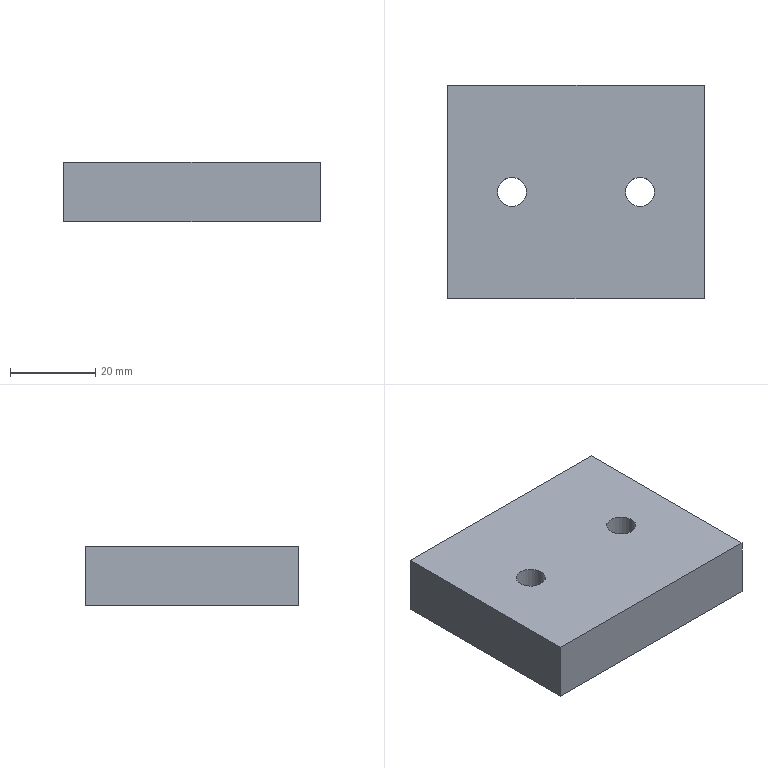Part | SolidWorks | features Extrusion 1, HoleWzd 1 | 1 solid | 10 faces | box 60 x 50 x 14 mm | volume 40983 mm3 | plane 6 | cylinder 4 | commonest cylinder face diameters 6.8 x4
STEP:
#1=CARTESIAN_POINT('',(-18.4,0.,0.));
#2=VERTEX_POINT('',#1);
#3=CARTESIAN_POINT('',(-11.6,0.,0.));
#4=VERTEX_POINT('',#3);
#5=CARTESIAN_POINT('',(-15.,0.,0.));
#6=DIRECTION('',(0.,0.,1.));
#7=DIRECTION('',(1.,0.,0.));
#8=AXIS2_PLACEMENT_3D('',#5,#6,#7);
#9=CIRCLE('',#8,3.4);
#10=EDGE_CURVE('',#2,#4,#9,.T.);
#11=ORIENTED_EDGE('',*,*,#10,.F.);
#12=CARTESIAN_POINT('',(-18.4,0.,14.));
#13=VERTEX_POINT('',#12);
#14=CARTESIAN_POINT('',(-18.4,0.,14.));
#15=DIRECTION('',(0.,0.,1.));
#16=VECTOR('',#15,1000.);
#17=LINE('',#14,#16);
#18=EDGE_CURVE('',#2,#13,#17,.T.);
#19=ORIENTED_EDGE('',*,*,#18,.T.);
#20=CARTESIAN_POINT('',(-11.6,0.,14.));
#21=VERTEX_POINT('',#20);
#22=CARTESIAN_POINT('',(-15.,0.,14.));
#23=DIRECTION('',(0.,0.,1.));
#24=DIRECTION('',(1.,0.,0.));
#25=AXIS2_PLACEMENT_3D('',#22,#23,#24);
#26=CIRCLE('',#25,3.4);
#27=EDGE_CURVE('',#13,#21,#26,.T.);
#28=ORIENTED_EDGE('',*,*,#27,.T.);
#29=CARTESIAN_POINT('',(-11.6,0.,14.));
#30=DIRECTION('',(0.,0.,1.));
#31=VECTOR('',#30,1000.);
#32=LINE('',#29,#31);
#33=EDGE_CURVE('',#4,#21,#32,.T.);
#34=ORIENTED_EDGE('',*,*,#33,.F.);
#35=EDGE_LOOP('',(#11,#19,#28,#34));
#36=FACE_OUTER_BOUND('',#35,.T.);
#37=CARTESIAN_POINT('',(-15.,0.,14.));
#38=DIRECTION('',(0.,0.,1.));
#39=DIRECTION('',(1.,0.,0.));
#40=AXIS2_PLACEMENT_3D('',#37,#38,#39);
#41=CYLINDRICAL_SURFACE('',#40,3.4);
#42=ADVANCED_FACE('',(#36),#41,.F.);
#43=CARTESIAN_POINT('',(11.6,0.,0.));
#44=VERTEX_POINT('',#43);
#45=CARTESIAN_POINT('',(18.4,0.,0.));
#46=VERTEX_POINT('',#45);
#47=CARTESIAN_POINT('',(15.,0.,0.));
#48=DIRECTION('',(0.,0.,1.));
#49=DIRECTION('',(1.,0.,0.));
#50=AXIS2_PLACEMENT_3D('',#47,#48,#49);
#51=CIRCLE('',#50,3.4);
#52=EDGE_CURVE('',#44,#46,#51,.T.);
#53=ORIENTED_EDGE('',*,*,#52,.F.);
#54=CARTESIAN_POINT('',(11.6,0.,14.));
#55=VERTEX_POINT('',#54);
#56=CARTESIAN_POINT('',(11.6,0.,14.));
#57=DIRECTION('',(0.,0.,1.));
#58=VECTOR('',#57,1000.);
#59=LINE('',#56,#58);
#60=EDGE_CURVE('',#44,#55,#59,.T.);
#61=ORIENTED_EDGE('',*,*,#60,.T.);
#62=CARTESIAN_POINT('',(18.4,0.,14.));
#63=VERTEX_POINT('',#62);
#64=CARTESIAN_POINT('',(15.,0.,14.));
#65=DIRECTION('',(0.,0.,1.));
#66=DIRECTION('',(1.,0.,0.));
#67=AXIS2_PLACEMENT_3D('',#64,#65,#66);
#68=CIRCLE('',#67,3.4);
#69=EDGE_CURVE('',#55,#63,#68,.T.);
#70=ORIENTED_EDGE('',*,*,#69,.T.);
#71=CARTESIAN_POINT('',(18.4,0.,14.));
#72=DIRECTION('',(0.,0.,1.));
#73=VECTOR('',#72,1000.);
#74=LINE('',#71,#73);
#75=EDGE_CURVE('',#46,#63,#74,.T.);
#76=ORIENTED_EDGE('',*,*,#75,.F.);
#77=EDGE_LOOP('',(#53,#61,#70,#76));
#78=FACE_OUTER_BOUND('',#77,.T.);
#79=CARTESIAN_POINT('',(15.,0.,14.));
#80=DIRECTION('',(0.,0.,1.));
#81=DIRECTION('',(1.,0.,0.));
#82=AXIS2_PLACEMENT_3D('',#79,#80,#81);
#83=CYLINDRICAL_SURFACE('',#82,3.4);
#84=ADVANCED_FACE('',(#78),#83,.F.);
#85=CARTESIAN_POINT('',(30.,-25.,0.));
#86=VERTEX_POINT('',#85);
#87=CARTESIAN_POINT('',(30.,25.,0.));
#88=VERTEX_POINT('',#87);
#89=CARTESIAN_POINT('',(30.,25.,0.));
#90=DIRECTION('',(0.,1.,0.));
#91=VECTOR('',#90,1000.);
#92=LINE('',#89,#91);
#93=EDGE_CURVE('',#86,#88,#92,.T.);
#94=ORIENTED_EDGE('',*,*,#93,.T.);
#95=CARTESIAN_POINT('',(30.,25.,14.));
#96=VERTEX_POINT('',#95);
#97=CARTESIAN_POINT('',(30.,25.,14.));
#98=DIRECTION('',(0.,0.,-1.));
#99=VECTOR('',#98,1000.);
#100=LINE('',#97,#99);
#101=EDGE_CURVE('',#96,#88,#100,.T.);
#102=ORIENTED_EDGE('',*,*,#101,.F.);
#103=CARTESIAN_POINT('',(30.,-25.,14.));
#104=VERTEX_POINT('',#103);
#105=CARTESIAN_POINT('',(30.,25.,14.));
#106=DIRECTION('',(0.,1.,0.));
#107=VECTOR('',#106,1000.);
#108=LINE('',#105,#107);
#109=EDGE_CURVE('',#104,#96,#108,.T.);
#110=ORIENTED_EDGE('',*,*,#109,.F.);
#111=CARTESIAN_POINT('',(30.,-25.,14.));
#112=DIRECTION('',(0.,0.,-1.));
#113=VECTOR('',#112,1000.);
#114=LINE('',#111,#113);
#115=EDGE_CURVE('',#104,#86,#114,.T.);
#116=ORIENTED_EDGE('',*,*,#115,.T.);
#117=EDGE_LOOP('',(#94,#102,#110,#116));
#118=FACE_OUTER_BOUND('',#117,.T.);
#119=CARTESIAN_POINT('',(30.,25.,14.));
#120=DIRECTION('',(-1.,0.,0.));
#121=DIRECTION('',(0.,-1.,0.));
#122=AXIS2_PLACEMENT_3D('',#119,#120,#121);
#123=PLANE('',#122);
#124=ADVANCED_FACE('',(#118),#123,.F.);
#125=CARTESIAN_POINT('',(-30.,25.,0.));
#126=VERTEX_POINT('',#125);
#127=CARTESIAN_POINT('',(-30.,25.,0.));
#128=DIRECTION('',(-1.,0.,0.));
#129=VECTOR('',#128,1000.);
#130=LINE('',#127,#129);
#131=EDGE_CURVE('',#88,#126,#130,.T.);
#132=ORIENTED_EDGE('',*,*,#131,.T.);
#133=CARTESIAN_POINT('',(-30.,25.,14.));
#134=VERTEX_POINT('',#133);
#135=CARTESIAN_POINT('',(-30.,25.,14.));
#136=DIRECTION('',(0.,0.,-1.));
#137=VECTOR('',#136,1000.);
#138=LINE('',#135,#137);
#139=EDGE_CURVE('',#134,#126,#138,.T.);
#140=ORIENTED_EDGE('',*,*,#139,.F.);
#141=CARTESIAN_POINT('',(-30.,25.,14.));
#142=DIRECTION('',(-1.,0.,0.));
#143=VECTOR('',#142,1000.);
#144=LINE('',#141,#143);
#145=EDGE_CURVE('',#96,#134,#144,.T.);
#146=ORIENTED_EDGE('',*,*,#145,.F.);
#147=ORIENTED_EDGE('',*,*,#101,.T.);
#148=EDGE_LOOP('',(#132,#140,#146,#147));
#149=FACE_OUTER_BOUND('',#148,.T.);
#150=CARTESIAN_POINT('',(-30.,25.,14.));
#151=DIRECTION('',(0.,-1.,0.));
#152=DIRECTION('',(0.,0.,-1.));
#153=AXIS2_PLACEMENT_3D('',#150,#151,#152);
#154=PLANE('',#153);
#155=ADVANCED_FACE('',(#149),#154,.F.);
#156=CARTESIAN_POINT('',(-30.,-25.,0.));
#157=VERTEX_POINT('',#156);
#158=CARTESIAN_POINT('',(-30.,25.,0.));
#159=DIRECTION('',(0.,-1.,0.));
#160=VECTOR('',#159,1000.);
#161=LINE('',#158,#160);
#162=EDGE_CURVE('',#126,#157,#161,.T.);
#163=ORIENTED_EDGE('',*,*,#162,.T.);
#164=CARTESIAN_POINT('',(-30.,-25.,14.));
#165=VERTEX_POINT('',#164);
#166=CARTESIAN_POINT('',(-30.,-25.,14.));
#167=DIRECTION('',(0.,0.,-1.));
#168=VECTOR('',#167,1000.);
#169=LINE('',#166,#168);
#170=EDGE_CURVE('',#165,#157,#169,.T.);
#171=ORIENTED_EDGE('',*,*,#170,.F.);
#172=CARTESIAN_POINT('',(-30.,25.,14.));
#173=DIRECTION('',(0.,-1.,0.));
#174=VECTOR('',#173,1000.);
#175=LINE('',#172,#174);
#176=EDGE_CURVE('',#134,#165,#175,.T.);
#177=ORIENTED_EDGE('',*,*,#176,.F.);
#178=ORIENTED_EDGE('',*,*,#139,.T.);
#179=EDGE_LOOP('',(#163,#171,#177,#178));
#180=FACE_OUTER_BOUND('',#179,.T.);
#181=CARTESIAN_POINT('',(-30.,25.,14.));
#182=DIRECTION('',(1.,0.,0.));
#183=DIRECTION('',(0.,1.,0.));
#184=AXIS2_PLACEMENT_3D('',#181,#182,#183);
#185=PLANE('',#184);
#186=ADVANCED_FACE('',(#180),#185,.F.);
#187=CARTESIAN_POINT('',(-30.,-25.,0.));
#188=DIRECTION('',(1.,0.,0.));
#189=VECTOR('',#188,1000.);
#190=LINE('',#187,#189);
#191=EDGE_CURVE('',#157,#86,#190,.T.);
#192=ORIENTED_EDGE('',*,*,#191,.T.);
#193=ORIENTED_EDGE('',*,*,#115,.F.);
#194=CARTESIAN_POINT('',(-30.,-25.,14.));
#195=DIRECTION('',(1.,0.,0.));
#196=VECTOR('',#195,1000.);
#197=LINE('',#194,#196);
#198=EDGE_CURVE('',#165,#104,#197,.T.);
#199=ORIENTED_EDGE('',*,*,#198,.F.);
#200=ORIENTED_EDGE('',*,*,#170,.T.);
#201=EDGE_LOOP('',(#192,#193,#199,#200));
#202=FACE_OUTER_BOUND('',#201,.T.);
#203=CARTESIAN_POINT('',(-30.,-25.,14.));
#204=DIRECTION('',(0.,1.,0.));
#205=DIRECTION('',(0.,0.,1.));
#206=AXIS2_PLACEMENT_3D('',#203,#204,#205);
#207=PLANE('',#206);
#208=ADVANCED_FACE('',(#202),#207,.F.);
#209=CARTESIAN_POINT('',(-15.,0.,14.));
#210=DIRECTION('',(0.,0.,1.));
#211=DIRECTION('',(1.,0.,0.));
#212=AXIS2_PLACEMENT_3D('',#209,#210,#211);
#213=CIRCLE('',#212,3.4);
#214=EDGE_CURVE('',#21,#13,#213,.T.);
#215=ORIENTED_EDGE('',*,*,#214,.F.);
#216=ORIENTED_EDGE('',*,*,#27,.F.);
#217=EDGE_LOOP('',(#215,#216));
#218=FACE_BOUND('',#217,.T.);
#219=CARTESIAN_POINT('',(15.,0.,14.));
#220=DIRECTION('',(0.,0.,1.));
#221=DIRECTION('',(1.,0.,0.));
#222=AXIS2_PLACEMENT_3D('',#219,#220,#221);
#223=CIRCLE('',#222,3.4);
#224=EDGE_CURVE('',#63,#55,#223,.T.);
#225=ORIENTED_EDGE('',*,*,#224,.F.);
#226=ORIENTED_EDGE('',*,*,#69,.F.);
#227=EDGE_LOOP('',(#225,#226));
#228=FACE_BOUND('',#227,.T.);
#229=ORIENTED_EDGE('',*,*,#109,.T.);
#230=ORIENTED_EDGE('',*,*,#145,.T.);
#231=ORIENTED_EDGE('',*,*,#176,.T.);
#232=ORIENTED_EDGE('',*,*,#198,.T.);
#233=EDGE_LOOP('',(#229,#230,#231,#232));
#234=FACE_OUTER_BOUND('',#233,.T.);
#235=CARTESIAN_POINT('',(0.,0.,14.));
#236=DIRECTION('',(0.,0.,1.));
#237=DIRECTION('',(1.,0.,0.));
#238=AXIS2_PLACEMENT_3D('',#235,#236,#237);
#239=PLANE('',#238);
#240=ADVANCED_FACE('',(#218,#228,#234),#239,.T.);
#241=CARTESIAN_POINT('',(-15.,0.,0.));
#242=DIRECTION('',(0.,0.,1.));
#243=DIRECTION('',(1.,0.,0.));
#244=AXIS2_PLACEMENT_3D('',#241,#242,#243);
#245=CIRCLE('',#244,3.4);
#246=EDGE_CURVE('',#4,#2,#245,.T.);
#247=ORIENTED_EDGE('',*,*,#246,.T.);
#248=ORIENTED_EDGE('',*,*,#10,.T.);
#249=EDGE_LOOP('',(#247,#248));
#250=FACE_BOUND('',#249,.T.);
#251=CARTESIAN_POINT('',(15.,0.,0.));
#252=DIRECTION('',(0.,0.,1.));
#253=DIRECTION('',(1.,0.,0.));
#254=AXIS2_PLACEMENT_3D('',#251,#252,#253);
#255=CIRCLE('',#254,3.4);
#256=EDGE_CURVE('',#46,#44,#255,.T.);
#257=ORIENTED_EDGE('',*,*,#256,.T.);
#258=ORIENTED_EDGE('',*,*,#52,.T.);
#259=EDGE_LOOP('',(#257,#258));
#260=FACE_BOUND('',#259,.T.);
#261=ORIENTED_EDGE('',*,*,#93,.F.);
#262=ORIENTED_EDGE('',*,*,#191,.F.);
#263=ORIENTED_EDGE('',*,*,#162,.F.);
#264=ORIENTED_EDGE('',*,*,#131,.F.);
#265=EDGE_LOOP('',(#261,#262,#263,#264));
#266=FACE_OUTER_BOUND('',#265,.T.);
#267=CARTESIAN_POINT('',(0.,0.,0.));
#268=DIRECTION('',(0.,0.,1.));
#269=DIRECTION('',(1.,0.,0.));
#270=AXIS2_PLACEMENT_3D('',#267,#268,#269);
#271=PLANE('',#270);
#272=ADVANCED_FACE('',(#250,#260,#266),#271,.F.);
#273=ORIENTED_EDGE('',*,*,#60,.F.);
#274=ORIENTED_EDGE('',*,*,#256,.F.);
#275=ORIENTED_EDGE('',*,*,#75,.T.);
#276=ORIENTED_EDGE('',*,*,#224,.T.);
#277=EDGE_LOOP('',(#273,#274,#275,#276));
#278=FACE_OUTER_BOUND('',#277,.T.);
#279=CARTESIAN_POINT('',(15.,0.,14.));
#280=DIRECTION('',(0.,0.,1.));
#281=DIRECTION('',(1.,0.,0.));
#282=AXIS2_PLACEMENT_3D('',#279,#280,#281);
#283=CYLINDRICAL_SURFACE('',#282,3.4);
#284=ADVANCED_FACE('',(#278),#283,.F.);
#285=ORIENTED_EDGE('',*,*,#18,.F.);
#286=ORIENTED_EDGE('',*,*,#246,.F.);
#287=ORIENTED_EDGE('',*,*,#33,.T.);
#288=ORIENTED_EDGE('',*,*,#214,.T.);
#289=EDGE_LOOP('',(#285,#286,#287,#288));
#290=FACE_OUTER_BOUND('',#289,.T.);
#291=CARTESIAN_POINT('',(-15.,0.,14.));
#292=DIRECTION('',(0.,0.,1.));
#293=DIRECTION('',(1.,0.,0.));
#294=AXIS2_PLACEMENT_3D('',#291,#292,#293);
#295=CYLINDRICAL_SURFACE('',#294,3.4);
#296=ADVANCED_FACE('',(#290),#295,.F.);
#297=CLOSED_SHELL('',(#42,#84,#124,#155,#186,#208,#240,#272,#284,#296));
#298=MANIFOLD_SOLID_BREP('',#297);
#299=CARTESIAN_POINT('',(0.,0.,0.));
#300=DIRECTION('',(0.,0.,1.));
#301=DIRECTION('',(1.,0.,0.));
#302=AXIS2_PLACEMENT_3D('',#299,#300,#301);
#303=(LENGTH_UNIT()NAMED_UNIT(*)SI_UNIT(.MILLI.,.METRE.));
#304=UNCERTAINTY_MEASURE_WITH_UNIT(LENGTH_MEASURE(0.00001),#303,'','');
#305=(NAMED_UNIT(*)PLANE_ANGLE_UNIT()SI_UNIT($,.RADIAN.));
#306=(NAMED_UNIT(*)SI_UNIT($,.STERADIAN.)SOLID_ANGLE_UNIT());
#307=(GEOMETRIC_REPRESENTATION_CONTEXT(3)GLOBAL_UNCERTAINTY_ASSIGNED_CONTEXT((#304))GLOBAL_UNIT_ASSIGNED_CONTEXT((#303,#305,#306))REPRESENTATION_CONTEXT('',''));
#308=ADVANCED_BREP_SHAPE_REPRESENTATION('',(#298,#302),#307);